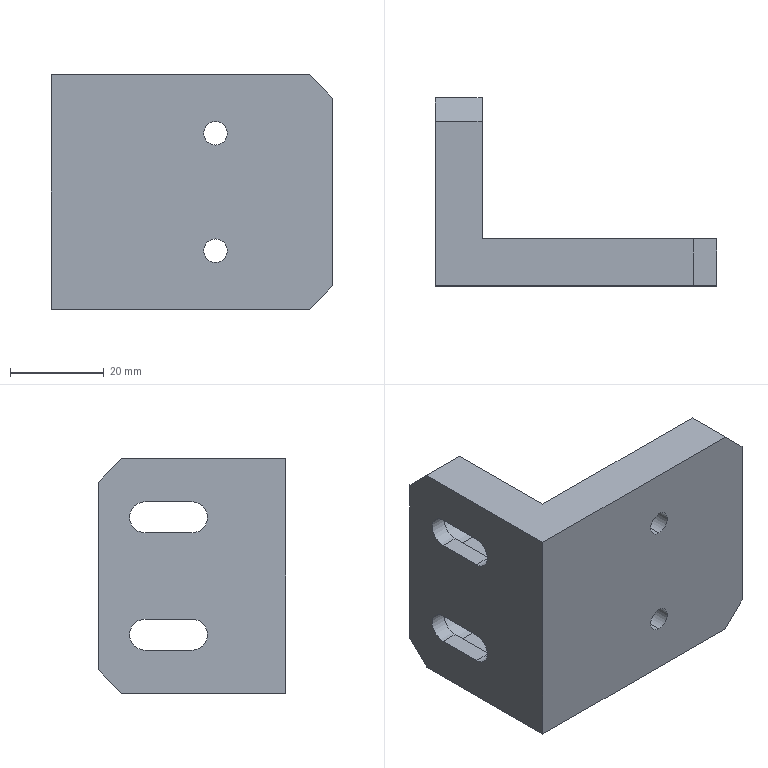Part | SolidWorks | features HoleWzd 2, Chamfer 1, Extrusion 1 | 1 solid | 34 faces | box 60 x 40 x 50 mm | volume 40761 mm3 | plane 22 | cylinder 12 | commonest cylinder face diameters 5 x4 6.6 x4 11 x4
STEP:
#1=CARTESIAN_POINT('',(25.,-10.,35.));
#2=VERTEX_POINT('',#1);
#3=CARTESIAN_POINT('',(25.,-10.,40.));
#4=VERTEX_POINT('',#3);
#5=CARTESIAN_POINT('',(25.,-10.,37.5));
#6=DIRECTION('',(0.,1.,0.));
#7=DIRECTION('',(-1.,0.,0.));
#8=AXIS2_PLACEMENT_3D('',#5,#6,#7);
#9=CIRCLE('',#8,2.5);
#10=EDGE_CURVE('',#2,#4,#9,.T.);
#11=ORIENTED_EDGE('',*,*,#10,.F.);
#12=CARTESIAN_POINT('',(25.,0.,35.));
#13=VERTEX_POINT('',#12);
#14=CARTESIAN_POINT('',(25.,0.,35.));
#15=DIRECTION('',(0.,1.,0.));
#16=VECTOR('',#15,1000.);
#17=LINE('',#14,#16);
#18=EDGE_CURVE('',#2,#13,#17,.T.);
#19=ORIENTED_EDGE('',*,*,#18,.T.);
#20=CARTESIAN_POINT('',(25.,0.,40.));
#21=VERTEX_POINT('',#20);
#22=CARTESIAN_POINT('',(25.,0.,37.5));
#23=DIRECTION('',(0.,1.,0.));
#24=DIRECTION('',(0.,0.,1.));
#25=AXIS2_PLACEMENT_3D('',#22,#23,#24);
#26=CIRCLE('',#25,2.5);
#27=EDGE_CURVE('',#13,#21,#26,.T.);
#28=ORIENTED_EDGE('',*,*,#27,.T.);
#29=CARTESIAN_POINT('',(25.,0.,40.));
#30=DIRECTION('',(0.,1.,0.));
#31=VECTOR('',#30,1000.);
#32=LINE('',#29,#31);
#33=EDGE_CURVE('',#4,#21,#32,.T.);
#34=ORIENTED_EDGE('',*,*,#33,.F.);
#35=EDGE_LOOP('',(#11,#19,#28,#34));
#36=FACE_OUTER_BOUND('',#35,.T.);
#37=CARTESIAN_POINT('',(25.,0.,37.5));
#38=DIRECTION('',(0.,1.,0.));
#39=DIRECTION('',(0.,0.,1.));
#40=AXIS2_PLACEMENT_3D('',#37,#38,#39);
#41=CYLINDRICAL_SURFACE('',#40,2.5);
#42=ADVANCED_FACE('',(#36),#41,.F.);
#43=CARTESIAN_POINT('',(25.,-10.,10.));
#44=VERTEX_POINT('',#43);
#45=CARTESIAN_POINT('',(25.,-10.,15.));
#46=VERTEX_POINT('',#45);
#47=CARTESIAN_POINT('',(25.,-10.,12.5));
#48=DIRECTION('',(0.,1.,0.));
#49=DIRECTION('',(-1.,0.,0.));
#50=AXIS2_PLACEMENT_3D('',#47,#48,#49);
#51=CIRCLE('',#50,2.5);
#52=EDGE_CURVE('',#44,#46,#51,.T.);
#53=ORIENTED_EDGE('',*,*,#52,.F.);
#54=CARTESIAN_POINT('',(25.,0.,10.));
#55=VERTEX_POINT('',#54);
#56=CARTESIAN_POINT('',(25.,0.,10.));
#57=DIRECTION('',(0.,1.,0.));
#58=VECTOR('',#57,1000.);
#59=LINE('',#56,#58);
#60=EDGE_CURVE('',#44,#55,#59,.T.);
#61=ORIENTED_EDGE('',*,*,#60,.T.);
#62=CARTESIAN_POINT('',(25.,0.,15.));
#63=VERTEX_POINT('',#62);
#64=CARTESIAN_POINT('',(25.,0.,12.5));
#65=DIRECTION('',(0.,1.,0.));
#66=DIRECTION('',(0.,0.,1.));
#67=AXIS2_PLACEMENT_3D('',#64,#65,#66);
#68=CIRCLE('',#67,2.5);
#69=EDGE_CURVE('',#55,#63,#68,.T.);
#70=ORIENTED_EDGE('',*,*,#69,.T.);
#71=CARTESIAN_POINT('',(25.,0.,15.));
#72=DIRECTION('',(0.,1.,0.));
#73=VECTOR('',#72,1000.);
#74=LINE('',#71,#73);
#75=EDGE_CURVE('',#46,#63,#74,.T.);
#76=ORIENTED_EDGE('',*,*,#75,.F.);
#77=EDGE_LOOP('',(#53,#61,#70,#76));
#78=FACE_OUTER_BOUND('',#77,.T.);
#79=CARTESIAN_POINT('',(25.,0.,12.5));
#80=DIRECTION('',(0.,1.,0.));
#81=DIRECTION('',(0.,0.,1.));
#82=AXIS2_PLACEMENT_3D('',#79,#80,#81);
#83=CYLINDRICAL_SURFACE('',#82,2.5);
#84=ADVANCED_FACE('',(#78),#83,.F.);
#85=CARTESIAN_POINT('',(0.,10.,32.));
#86=VERTEX_POINT('',#85);
#87=CARTESIAN_POINT('',(0.,20.,32.));
#88=VERTEX_POINT('',#87);
#89=CARTESIAN_POINT('',(0.,10.,32.));
#90=DIRECTION('',(0.,1.,0.));
#91=VECTOR('',#90,1000.);
#92=LINE('',#89,#91);
#93=EDGE_CURVE('',#86,#88,#92,.T.);
#94=ORIENTED_EDGE('',*,*,#93,.F.);
#95=CARTESIAN_POINT('',(0.,10.,43.));
#96=VERTEX_POINT('',#95);
#97=CARTESIAN_POINT('',(0.,10.,37.5));
#98=DIRECTION('',(1.,0.,0.));
#99=DIRECTION('',(0.,0.,-1.));
#100=AXIS2_PLACEMENT_3D('',#97,#98,#99);
#101=CIRCLE('',#100,5.5);
#102=EDGE_CURVE('',#96,#86,#101,.T.);
#103=ORIENTED_EDGE('',*,*,#102,.F.);
#104=CARTESIAN_POINT('',(0.,20.,43.));
#105=VERTEX_POINT('',#104);
#106=CARTESIAN_POINT('',(0.,10.,43.));
#107=DIRECTION('',(0.,1.,0.));
#108=VECTOR('',#107,1000.);
#109=LINE('',#106,#108);
#110=EDGE_CURVE('',#96,#105,#109,.T.);
#111=ORIENTED_EDGE('',*,*,#110,.T.);
#112=CARTESIAN_POINT('',(0.,20.,37.5));
#113=DIRECTION('',(1.,0.,0.));
#114=DIRECTION('',(0.,0.,-1.));
#115=AXIS2_PLACEMENT_3D('',#112,#113,#114);
#116=CIRCLE('',#115,5.5);
#117=EDGE_CURVE('',#88,#105,#116,.T.);
#118=ORIENTED_EDGE('',*,*,#117,.F.);
#119=EDGE_LOOP('',(#94,#103,#111,#118));
#120=FACE_BOUND('',#119,.T.);
#121=CARTESIAN_POINT('',(0.,30.,45.));
#122=VERTEX_POINT('',#121);
#123=CARTESIAN_POINT('',(0.,30.,5.));
#124=VERTEX_POINT('',#123);
#125=CARTESIAN_POINT('',(0.,30.,50.));
#126=DIRECTION('',(0.,0.,-1.));
#127=VECTOR('',#126,1000.);
#128=LINE('',#125,#127);
#129=EDGE_CURVE('',#122,#124,#128,.T.);
#130=ORIENTED_EDGE('',*,*,#129,.F.);
#131=CARTESIAN_POINT('',(0.,25.,50.));
#132=VERTEX_POINT('',#131);
#133=CARTESIAN_POINT('',(0.,25.,50.));
#134=DIRECTION('',(0.,-0.7071,0.7071));
#135=VECTOR('',#134,1000.);
#136=LINE('',#133,#135);
#137=EDGE_CURVE('',#122,#132,#136,.T.);
#138=ORIENTED_EDGE('',*,*,#137,.T.);
#139=CARTESIAN_POINT('',(0.,0.,50.));
#140=VERTEX_POINT('',#139);
#141=CARTESIAN_POINT('',(0.,0.,50.));
#142=DIRECTION('',(0.,1.,0.));
#143=VECTOR('',#142,1000.);
#144=LINE('',#141,#143);
#145=EDGE_CURVE('',#140,#132,#144,.T.);
#146=ORIENTED_EDGE('',*,*,#145,.F.);
#147=CARTESIAN_POINT('',(0.,0.,0.));
#148=VERTEX_POINT('',#147);
#149=CARTESIAN_POINT('',(0.,0.,50.));
#150=DIRECTION('',(0.,0.,-1.));
#151=VECTOR('',#150,1000.);
#152=LINE('',#149,#151);
#153=EDGE_CURVE('',#140,#148,#152,.T.);
#154=ORIENTED_EDGE('',*,*,#153,.T.);
#155=CARTESIAN_POINT('',(0.,25.,0.));
#156=VERTEX_POINT('',#155);
#157=CARTESIAN_POINT('',(0.,0.,0.));
#158=DIRECTION('',(0.,1.,0.));
#159=VECTOR('',#158,1000.);
#160=LINE('',#157,#159);
#161=EDGE_CURVE('',#148,#156,#160,.T.);
#162=ORIENTED_EDGE('',*,*,#161,.T.);
#163=CARTESIAN_POINT('',(0.,30.,5.));
#164=DIRECTION('',(0.,0.7071,0.7071));
#165=VECTOR('',#164,1000.);
#166=LINE('',#163,#165);
#167=EDGE_CURVE('',#156,#124,#166,.T.);
#168=ORIENTED_EDGE('',*,*,#167,.T.);
#169=EDGE_LOOP('',(#130,#138,#146,#154,#162,#168));
#170=FACE_OUTER_BOUND('',#169,.T.);
#171=CARTESIAN_POINT('',(0.,10.,7.));
#172=VERTEX_POINT('',#171);
#173=CARTESIAN_POINT('',(0.,20.,7.));
#174=VERTEX_POINT('',#173);
#175=CARTESIAN_POINT('',(0.,10.,7.));
#176=DIRECTION('',(0.,1.,0.));
#177=VECTOR('',#176,1000.);
#178=LINE('',#175,#177);
#179=EDGE_CURVE('',#172,#174,#178,.T.);
#180=ORIENTED_EDGE('',*,*,#179,.F.);
#181=CARTESIAN_POINT('',(0.,10.,18.));
#182=VERTEX_POINT('',#181);
#183=CARTESIAN_POINT('',(0.,10.,12.5));
#184=DIRECTION('',(1.,0.,0.));
#185=DIRECTION('',(0.,0.,-1.));
#186=AXIS2_PLACEMENT_3D('',#183,#184,#185);
#187=CIRCLE('',#186,5.5);
#188=EDGE_CURVE('',#182,#172,#187,.T.);
#189=ORIENTED_EDGE('',*,*,#188,.F.);
#190=CARTESIAN_POINT('',(0.,20.,18.));
#191=VERTEX_POINT('',#190);
#192=CARTESIAN_POINT('',(0.,10.,18.));
#193=DIRECTION('',(0.,1.,0.));
#194=VECTOR('',#193,1000.);
#195=LINE('',#192,#194);
#196=EDGE_CURVE('',#182,#191,#195,.T.);
#197=ORIENTED_EDGE('',*,*,#196,.T.);
#198=CARTESIAN_POINT('',(0.,20.,12.5));
#199=DIRECTION('',(1.,0.,0.));
#200=DIRECTION('',(0.,0.,-1.));
#201=AXIS2_PLACEMENT_3D('',#198,#199,#200);
#202=CIRCLE('',#201,5.5);
#203=EDGE_CURVE('',#174,#191,#202,.T.);
#204=ORIENTED_EDGE('',*,*,#203,.F.);
#205=EDGE_LOOP('',(#180,#189,#197,#204));
#206=FACE_BOUND('',#205,.T.);
#207=CARTESIAN_POINT('',(0.,0.,50.));
#208=DIRECTION('',(-1.,0.,0.));
#209=DIRECTION('',(0.,-1.,0.));
#210=AXIS2_PLACEMENT_3D('',#207,#208,#209);
#211=PLANE('',#210);
#212=ADVANCED_FACE('',(#120,#170,#206),#211,.F.);
#213=CARTESIAN_POINT('',(50.,-10.,45.));
#214=VERTEX_POINT('',#213);
#215=CARTESIAN_POINT('',(50.,-10.,5.));
#216=VERTEX_POINT('',#215);
#217=CARTESIAN_POINT('',(50.,-10.,50.));
#218=DIRECTION('',(0.,0.,-1.));
#219=VECTOR('',#218,1000.);
#220=LINE('',#217,#219);
#221=EDGE_CURVE('',#214,#216,#220,.T.);
#222=ORIENTED_EDGE('',*,*,#221,.T.);
#223=CARTESIAN_POINT('',(50.,0.,5.));
#224=VERTEX_POINT('',#223);
#225=CARTESIAN_POINT('',(50.,0.,5.));
#226=DIRECTION('',(0.,1.,0.));
#227=VECTOR('',#226,1000.);
#228=LINE('',#225,#227);
#229=EDGE_CURVE('',#216,#224,#228,.T.);
#230=ORIENTED_EDGE('',*,*,#229,.T.);
#231=CARTESIAN_POINT('',(50.,0.,45.));
#232=VERTEX_POINT('',#231);
#233=CARTESIAN_POINT('',(50.,0.,50.));
#234=DIRECTION('',(0.,0.,-1.));
#235=VECTOR('',#234,1000.);
#236=LINE('',#233,#235);
#237=EDGE_CURVE('',#232,#224,#236,.T.);
#238=ORIENTED_EDGE('',*,*,#237,.F.);
#239=CARTESIAN_POINT('',(50.,0.,45.));
#240=DIRECTION('',(0.,-1.,0.));
#241=VECTOR('',#240,1000.);
#242=LINE('',#239,#241);
#243=EDGE_CURVE('',#232,#214,#242,.T.);
#244=ORIENTED_EDGE('',*,*,#243,.T.);
#245=EDGE_LOOP('',(#222,#230,#238,#244));
#246=FACE_OUTER_BOUND('',#245,.T.);
#247=CARTESIAN_POINT('',(50.,0.,50.));
#248=DIRECTION('',(-1.,0.,0.));
#249=DIRECTION('',(0.,0.,1.));
#250=AXIS2_PLACEMENT_3D('',#247,#248,#249);
#251=PLANE('',#250);
#252=ADVANCED_FACE('',(#246),#251,.F.);
#253=CARTESIAN_POINT('',(25.,0.,37.5));
#254=DIRECTION('',(0.,1.,0.));
#255=DIRECTION('',(0.,0.,1.));
#256=AXIS2_PLACEMENT_3D('',#253,#254,#255);
#257=CIRCLE('',#256,2.5);
#258=EDGE_CURVE('',#21,#13,#257,.T.);
#259=ORIENTED_EDGE('',*,*,#258,.F.);
#260=ORIENTED_EDGE('',*,*,#27,.F.);
#261=EDGE_LOOP('',(#259,#260));
#262=FACE_BOUND('',#261,.T.);
#263=CARTESIAN_POINT('',(25.,0.,12.5));
#264=DIRECTION('',(0.,1.,0.));
#265=DIRECTION('',(0.,0.,1.));
#266=AXIS2_PLACEMENT_3D('',#263,#264,#265);
#267=CIRCLE('',#266,2.5);
#268=EDGE_CURVE('',#63,#55,#267,.T.);
#269=ORIENTED_EDGE('',*,*,#268,.F.);
#270=ORIENTED_EDGE('',*,*,#69,.F.);
#271=EDGE_LOOP('',(#269,#270));
#272=FACE_BOUND('',#271,.T.);
#273=ORIENTED_EDGE('',*,*,#237,.T.);
#274=CARTESIAN_POINT('',(45.,0.,0.));
#275=VERTEX_POINT('',#274);
#276=CARTESIAN_POINT('',(50.,0.,5.));
#277=DIRECTION('',(-0.7071,0.,-0.7071));
#278=VECTOR('',#277,1000.);
#279=LINE('',#276,#278);
#280=EDGE_CURVE('',#224,#275,#279,.T.);
#281=ORIENTED_EDGE('',*,*,#280,.T.);
#282=CARTESIAN_POINT('',(50.,0.,0.));
#283=DIRECTION('',(-1.,0.,0.));
#284=VECTOR('',#283,1000.);
#285=LINE('',#282,#284);
#286=EDGE_CURVE('',#275,#148,#285,.T.);
#287=ORIENTED_EDGE('',*,*,#286,.T.);
#288=ORIENTED_EDGE('',*,*,#153,.F.);
#289=CARTESIAN_POINT('',(45.,0.,50.));
#290=VERTEX_POINT('',#289);
#291=CARTESIAN_POINT('',(50.,0.,50.));
#292=DIRECTION('',(-1.,0.,0.));
#293=VECTOR('',#292,1000.);
#294=LINE('',#291,#293);
#295=EDGE_CURVE('',#290,#140,#294,.T.);
#296=ORIENTED_EDGE('',*,*,#295,.F.);
#297=CARTESIAN_POINT('',(45.,0.,50.));
#298=DIRECTION('',(0.7071,0.,-0.7071));
#299=VECTOR('',#298,1000.);
#300=LINE('',#297,#299);
#301=EDGE_CURVE('',#290,#232,#300,.T.);
#302=ORIENTED_EDGE('',*,*,#301,.T.);
#303=EDGE_LOOP('',(#273,#281,#287,#288,#296,#302));
#304=FACE_OUTER_BOUND('',#303,.T.);
#305=CARTESIAN_POINT('',(50.,0.,50.));
#306=DIRECTION('',(0.,-1.,0.));
#307=DIRECTION('',(1.,0.,0.));
#308=AXIS2_PLACEMENT_3D('',#305,#306,#307);
#309=PLANE('',#308);
#310=ADVANCED_FACE('',(#262,#272,#304),#309,.F.);
#311=CARTESIAN_POINT('',(-10.,30.,45.));
#312=VERTEX_POINT('',#311);
#313=CARTESIAN_POINT('',(-10.,30.,5.));
#314=VERTEX_POINT('',#313);
#315=CARTESIAN_POINT('',(-10.,30.,50.));
#316=DIRECTION('',(0.,0.,-1.));
#317=VECTOR('',#316,1000.);
#318=LINE('',#315,#317);
#319=EDGE_CURVE('',#312,#314,#318,.T.);
#320=ORIENTED_EDGE('',*,*,#319,.F.);
#321=CARTESIAN_POINT('',(-10.,30.,45.));
#322=DIRECTION('',(1.,0.,0.));
#323=VECTOR('',#322,1000.);
#324=LINE('',#321,#323);
#325=EDGE_CURVE('',#312,#122,#324,.T.);
#326=ORIENTED_EDGE('',*,*,#325,.T.);
#327=ORIENTED_EDGE('',*,*,#129,.T.);
#328=CARTESIAN_POINT('',(-10.,30.,5.));
#329=DIRECTION('',(-1.,0.,0.));
#330=VECTOR('',#329,1000.);
#331=LINE('',#328,#330);
#332=EDGE_CURVE('',#124,#314,#331,.T.);
#333=ORIENTED_EDGE('',*,*,#332,.T.);
#334=EDGE_LOOP('',(#320,#326,#327,#333));
#335=FACE_OUTER_BOUND('',#334,.T.);
#336=CARTESIAN_POINT('',(-10.,30.,50.));
#337=DIRECTION('',(0.,-1.,0.));
#338=DIRECTION('',(1.,0.,0.));
#339=AXIS2_PLACEMENT_3D('',#336,#337,#338);
#340=PLANE('',#339);
#341=ADVANCED_FACE('',(#335),#340,.F.);
#342=CARTESIAN_POINT('',(-10.,10.,34.2));
#343=VERTEX_POINT('',#342);
#344=CARTESIAN_POINT('',(-10.,20.,34.2));
#345=VERTEX_POINT('',#344);
#346=CARTESIAN_POINT('',(-10.,-10.,34.2));
#347=DIRECTION('',(0.,1.,0.));
#348=VECTOR('',#347,1000.);
#349=LINE('',#346,#348);
#350=EDGE_CURVE('',#343,#345,#349,.T.);
#351=ORIENTED_EDGE('',*,*,#350,.T.);
#352=CARTESIAN_POINT('',(-10.,20.,40.8));
#353=VERTEX_POINT('',#352);
#354=CARTESIAN_POINT('',(-10.,20.,37.5));
#355=DIRECTION('',(1.,0.,0.));
#356=DIRECTION('',(0.,1.,0.));
#357=AXIS2_PLACEMENT_3D('',#354,#355,#356);
#358=CIRCLE('',#357,3.3);
#359=EDGE_CURVE('',#345,#353,#358,.T.);
#360=ORIENTED_EDGE('',*,*,#359,.T.);
#361=CARTESIAN_POINT('',(-10.,10.,40.8));
#362=VERTEX_POINT('',#361);
#363=CARTESIAN_POINT('',(-10.,-10.,40.8));
#364=DIRECTION('',(0.,-1.,0.));
#365=VECTOR('',#364,1000.);
#366=LINE('',#363,#365);
#367=EDGE_CURVE('',#353,#362,#366,.T.);
#368=ORIENTED_EDGE('',*,*,#367,.T.);
#369=CARTESIAN_POINT('',(-10.,10.,37.5));
#370=DIRECTION('',(1.,0.,0.));
#371=DIRECTION('',(0.,1.,0.));
#372=AXIS2_PLACEMENT_3D('',#369,#370,#371);
#373=CIRCLE('',#372,3.3);
#374=EDGE_CURVE('',#362,#343,#373,.T.);
#375=ORIENTED_EDGE('',*,*,#374,.T.);
#376=EDGE_LOOP('',(#351,#360,#368,#375));
#377=FACE_BOUND('',#376,.T.);
#378=CARTESIAN_POINT('',(-10.,20.,15.8));
#379=VERTEX_POINT('',#378);
#380=CARTESIAN_POINT('',(-10.,10.,15.8));
#381=VERTEX_POINT('',#380);
#382=CARTESIAN_POINT('',(-10.,-10.,15.8));
#383=DIRECTION('',(0.,-1.,0.));
#384=VECTOR('',#383,1000.);
#385=LINE('',#382,#384);
#386=EDGE_CURVE('',#379,#381,#385,.T.);
#387=ORIENTED_EDGE('',*,*,#386,.T.);
#388=CARTESIAN_POINT('',(-10.,10.,9.2));
#389=VERTEX_POINT('',#388);
#390=CARTESIAN_POINT('',(-10.,10.,12.5));
#391=DIRECTION('',(1.,0.,0.));
#392=DIRECTION('',(0.,1.,0.));
#393=AXIS2_PLACEMENT_3D('',#390,#391,#392);
#394=CIRCLE('',#393,3.3);
#395=EDGE_CURVE('',#381,#389,#394,.T.);
#396=ORIENTED_EDGE('',*,*,#395,.T.);
#397=CARTESIAN_POINT('',(-10.,20.,9.2));
#398=VERTEX_POINT('',#397);
#399=CARTESIAN_POINT('',(-10.,-10.,9.2));
#400=DIRECTION('',(0.,1.,0.));
#401=VECTOR('',#400,1000.);
#402=LINE('',#399,#401);
#403=EDGE_CURVE('',#389,#398,#402,.T.);
#404=ORIENTED_EDGE('',*,*,#403,.T.);
#405=CARTESIAN_POINT('',(-10.,20.,12.5));
#406=DIRECTION('',(1.,0.,0.));
#407=DIRECTION('',(0.,1.,0.));
#408=AXIS2_PLACEMENT_3D('',#405,#406,#407);
#409=CIRCLE('',#408,3.3);
#410=EDGE_CURVE('',#398,#379,#409,.T.);
#411=ORIENTED_EDGE('',*,*,#410,.T.);
#412=EDGE_LOOP('',(#387,#396,#404,#411));
#413=FACE_BOUND('',#412,.T.);
#414=CARTESIAN_POINT('',(-10.,25.,50.));
#415=VERTEX_POINT('',#414);
#416=CARTESIAN_POINT('',(-10.,-10.,50.));
#417=VERTEX_POINT('',#416);
#418=CARTESIAN_POINT('',(-10.,-10.,50.));
#419=DIRECTION('',(0.,-1.,0.));
#420=VECTOR('',#419,1000.);
#421=LINE('',#418,#420);
#422=EDGE_CURVE('',#415,#417,#421,.T.);
#423=ORIENTED_EDGE('',*,*,#422,.F.);
#424=CARTESIAN_POINT('',(-10.,25.,50.));
#425=DIRECTION('',(0.,0.7071,-0.7071));
#426=VECTOR('',#425,1000.);
#427=LINE('',#424,#426);
#428=EDGE_CURVE('',#415,#312,#427,.T.);
#429=ORIENTED_EDGE('',*,*,#428,.T.);
#430=ORIENTED_EDGE('',*,*,#319,.T.);
#431=CARTESIAN_POINT('',(-10.,25.,0.));
#432=VERTEX_POINT('',#431);
#433=CARTESIAN_POINT('',(-10.,30.,5.));
#434=DIRECTION('',(0.,-0.7071,-0.7071));
#435=VECTOR('',#434,1000.);
#436=LINE('',#433,#435);
#437=EDGE_CURVE('',#314,#432,#436,.T.);
#438=ORIENTED_EDGE('',*,*,#437,.T.);
#439=CARTESIAN_POINT('',(-10.,-10.,0.));
#440=VERTEX_POINT('',#439);
#441=CARTESIAN_POINT('',(-10.,-10.,0.));
#442=DIRECTION('',(0.,-1.,0.));
#443=VECTOR('',#442,1000.);
#444=LINE('',#441,#443);
#445=EDGE_CURVE('',#432,#440,#444,.T.);
#446=ORIENTED_EDGE('',*,*,#445,.T.);
#447=CARTESIAN_POINT('',(-10.,-10.,50.));
#448=DIRECTION('',(0.,0.,-1.));
#449=VECTOR('',#448,1000.);
#450=LINE('',#447,#449);
#451=EDGE_CURVE('',#417,#440,#450,.T.);
#452=ORIENTED_EDGE('',*,*,#451,.F.);
#453=EDGE_LOOP('',(#423,#429,#430,#438,#446,#452));
#454=FACE_OUTER_BOUND('',#453,.T.);
#455=CARTESIAN_POINT('',(-10.,-10.,50.));
#456=DIRECTION('',(1.,0.,0.));
#457=DIRECTION('',(0.,1.,0.));
#458=AXIS2_PLACEMENT_3D('',#455,#456,#457);
#459=PLANE('',#458);
#460=ADVANCED_FACE('',(#377,#413,#454),#459,.F.);
#461=CARTESIAN_POINT('',(25.,-10.,37.5));
#462=DIRECTION('',(0.,1.,0.));
#463=DIRECTION('',(-1.,0.,0.));
#464=AXIS2_PLACEMENT_3D('',#461,#462,#463);
#465=CIRCLE('',#464,2.5);
#466=EDGE_CURVE('',#4,#2,#465,.T.);
#467=ORIENTED_EDGE('',*,*,#466,.T.);
#468=ORIENTED_EDGE('',*,*,#10,.T.);
#469=EDGE_LOOP('',(#467,#468));
#470=FACE_BOUND('',#469,.T.);
#471=CARTESIAN_POINT('',(25.,-10.,12.5));
#472=DIRECTION('',(0.,1.,0.));
#473=DIRECTION('',(-1.,0.,0.));
#474=AXIS2_PLACEMENT_3D('',#471,#472,#473);
#475=CIRCLE('',#474,2.5);
#476=EDGE_CURVE('',#46,#44,#475,.T.);
#477=ORIENTED_EDGE('',*,*,#476,.T.);
#478=ORIENTED_EDGE('',*,*,#52,.T.);
#479=EDGE_LOOP('',(#477,#478));
#480=FACE_BOUND('',#479,.T.);
#481=CARTESIAN_POINT('',(45.,-10.,0.));
#482=VERTEX_POINT('',#481);
#483=CARTESIAN_POINT('',(50.,-10.,0.));
#484=DIRECTION('',(1.,0.,0.));
#485=VECTOR('',#484,1000.);
#486=LINE('',#483,#485);
#487=EDGE_CURVE('',#440,#482,#486,.T.);
#488=ORIENTED_EDGE('',*,*,#487,.T.);
#489=CARTESIAN_POINT('',(50.,-10.,5.));
#490=DIRECTION('',(0.7071,0.,0.7071));
#491=VECTOR('',#490,1000.);
#492=LINE('',#489,#491);
#493=EDGE_CURVE('',#482,#216,#492,.T.);
#494=ORIENTED_EDGE('',*,*,#493,.T.);
#495=ORIENTED_EDGE('',*,*,#221,.F.);
#496=CARTESIAN_POINT('',(45.,-10.,50.));
#497=VERTEX_POINT('',#496);
#498=CARTESIAN_POINT('',(45.,-10.,50.));
#499=DIRECTION('',(-0.7071,0.,0.7071));
#500=VECTOR('',#499,1000.);
#501=LINE('',#498,#500);
#502=EDGE_CURVE('',#214,#497,#501,.T.);
#503=ORIENTED_EDGE('',*,*,#502,.T.);
#504=CARTESIAN_POINT('',(50.,-10.,50.));
#505=DIRECTION('',(1.,0.,0.));
#506=VECTOR('',#505,1000.);
#507=LINE('',#504,#506);
#508=EDGE_CURVE('',#417,#497,#507,.T.);
#509=ORIENTED_EDGE('',*,*,#508,.F.);
#510=ORIENTED_EDGE('',*,*,#451,.T.);
#511=EDGE_LOOP('',(#488,#494,#495,#503,#509,#510));
#512=FACE_OUTER_BOUND('',#511,.T.);
#513=CARTESIAN_POINT('',(50.,-10.,50.));
#514=DIRECTION('',(0.,1.,0.));
#515=DIRECTION('',(-1.,0.,0.));
#516=AXIS2_PLACEMENT_3D('',#513,#514,#515);
#517=PLANE('',#516);
#518=ADVANCED_FACE('',(#470,#480,#512),#517,.F.);
#519=ORIENTED_EDGE('',*,*,#508,.T.);
#520=CARTESIAN_POINT('',(45.,0.,50.));
#521=DIRECTION('',(0.,1.,0.));
#522=VECTOR('',#521,1000.);
#523=LINE('',#520,#522);
#524=EDGE_CURVE('',#497,#290,#523,.T.);
#525=ORIENTED_EDGE('',*,*,#524,.T.);
#526=ORIENTED_EDGE('',*,*,#295,.T.);
#527=ORIENTED_EDGE('',*,*,#145,.T.);
#528=CARTESIAN_POINT('',(0.,25.,50.));
#529=DIRECTION('',(-1.,0.,0.));
#530=VECTOR('',#529,1000.);
#531=LINE('',#528,#530);
#532=EDGE_CURVE('',#132,#415,#531,.T.);
#533=ORIENTED_EDGE('',*,*,#532,.T.);
#534=ORIENTED_EDGE('',*,*,#422,.T.);
#535=EDGE_LOOP('',(#519,#525,#526,#527,#533,#534));
#536=FACE_OUTER_BOUND('',#535,.T.);
#537=CARTESIAN_POINT('',(0.,0.,50.));
#538=DIRECTION('',(0.,0.,-1.));
#539=DIRECTION('',(-1.,0.,0.));
#540=AXIS2_PLACEMENT_3D('',#537,#538,#539);
#541=PLANE('',#540);
#542=ADVANCED_FACE('',(#536),#541,.F.);
#543=ORIENTED_EDGE('',*,*,#286,.F.);
#544=CARTESIAN_POINT('',(45.,-10.,0.));
#545=DIRECTION('',(0.,-1.,0.));
#546=VECTOR('',#545,1000.);
#547=LINE('',#544,#546);
#548=EDGE_CURVE('',#275,#482,#547,.T.);
#549=ORIENTED_EDGE('',*,*,#548,.T.);
#550=ORIENTED_EDGE('',*,*,#487,.F.);
#551=ORIENTED_EDGE('',*,*,#445,.F.);
#552=CARTESIAN_POINT('',(0.,25.,0.));
#553=DIRECTION('',(1.,0.,0.));
#554=VECTOR('',#553,1000.);
#555=LINE('',#552,#554);
#556=EDGE_CURVE('',#432,#156,#555,.T.);
#557=ORIENTED_EDGE('',*,*,#556,.T.);
#558=ORIENTED_EDGE('',*,*,#161,.F.);
#559=EDGE_LOOP('',(#543,#549,#550,#551,#557,#558));
#560=FACE_OUTER_BOUND('',#559,.T.);
#561=CARTESIAN_POINT('',(0.,0.,0.));
#562=DIRECTION('',(0.,0.,-1.));
#563=DIRECTION('',(-1.,0.,0.));
#564=AXIS2_PLACEMENT_3D('',#561,#562,#563);
#565=PLANE('',#564);
#566=ADVANCED_FACE('',(#560),#565,.T.);
#567=CARTESIAN_POINT('',(-6.4,10.,15.8));
#568=VERTEX_POINT('',#567);
#569=CARTESIAN_POINT('',(0.,10.,15.8));
#570=DIRECTION('',(-1.,0.,0.));
#571=VECTOR('',#570,1000.);
#572=LINE('',#569,#571);
#573=EDGE_CURVE('',#568,#381,#572,.T.);
#574=ORIENTED_EDGE('',*,*,#573,.F.);
#575=CARTESIAN_POINT('',(-6.4,10.,9.2));
#576=VERTEX_POINT('',#575);
#577=CARTESIAN_POINT('',(-6.4,10.,12.5));
#578=DIRECTION('',(1.,0.,0.));
#579=DIRECTION('',(0.,0.,-1.));
#580=AXIS2_PLACEMENT_3D('',#577,#578,#579);
#581=CIRCLE('',#580,3.3);
#582=EDGE_CURVE('',#568,#576,#581,.T.);
#583=ORIENTED_EDGE('',*,*,#582,.T.);
#584=CARTESIAN_POINT('',(0.,10.,9.2));
#585=DIRECTION('',(1.,0.,0.));
#586=VECTOR('',#585,1000.);
#587=LINE('',#584,#586);
#588=EDGE_CURVE('',#389,#576,#587,.T.);
#589=ORIENTED_EDGE('',*,*,#588,.F.);
#590=ORIENTED_EDGE('',*,*,#395,.F.);
#591=EDGE_LOOP('',(#574,#583,#589,#590));
#592=FACE_OUTER_BOUND('',#591,.T.);
#593=CARTESIAN_POINT('',(0.,10.,12.5));
#594=DIRECTION('',(1.,0.,0.));
#595=DIRECTION('',(0.,0.,-1.));
#596=AXIS2_PLACEMENT_3D('',#593,#594,#595);
#597=CYLINDRICAL_SURFACE('',#596,3.3);
#598=ADVANCED_FACE('',(#592),#597,.F.);
#599=CARTESIAN_POINT('',(-6.4,20.,15.8));
#600=VERTEX_POINT('',#599);
#601=CARTESIAN_POINT('',(0.,20.,15.8));
#602=DIRECTION('',(1.,0.,0.));
#603=VECTOR('',#602,1000.);
#604=LINE('',#601,#603);
#605=EDGE_CURVE('',#379,#600,#604,.T.);
#606=ORIENTED_EDGE('',*,*,#605,.T.);
#607=CARTESIAN_POINT('',(-6.4,10.,15.8));
#608=DIRECTION('',(0.,1.,0.));
#609=VECTOR('',#608,1000.);
#610=LINE('',#607,#609);
#611=EDGE_CURVE('',#568,#600,#610,.T.);
#612=ORIENTED_EDGE('',*,*,#611,.F.);
#613=ORIENTED_EDGE('',*,*,#573,.T.);
#614=ORIENTED_EDGE('',*,*,#386,.F.);
#615=EDGE_LOOP('',(#606,#612,#613,#614));
#616=FACE_OUTER_BOUND('',#615,.T.);
#617=CARTESIAN_POINT('',(0.,10.,15.8));
#618=DIRECTION('',(0.,0.,1.));
#619=DIRECTION('',(1.,0.,0.));
#620=AXIS2_PLACEMENT_3D('',#617,#618,#619);
#621=PLANE('',#620);
#622=ADVANCED_FACE('',(#616),#621,.F.);
#623=CARTESIAN_POINT('',(-6.4,20.,9.2));
#624=VERTEX_POINT('',#623);
#625=CARTESIAN_POINT('',(0.,20.,9.2));
#626=DIRECTION('',(-1.,0.,0.));
#627=VECTOR('',#626,1000.);
#628=LINE('',#625,#627);
#629=EDGE_CURVE('',#624,#398,#628,.T.);
#630=ORIENTED_EDGE('',*,*,#629,.F.);
#631=CARTESIAN_POINT('',(-6.4,20.,12.5));
#632=DIRECTION('',(1.,0.,0.));
#633=DIRECTION('',(0.,0.,-1.));
#634=AXIS2_PLACEMENT_3D('',#631,#632,#633);
#635=CIRCLE('',#634,3.3);
#636=EDGE_CURVE('',#624,#600,#635,.T.);
#637=ORIENTED_EDGE('',*,*,#636,.T.);
#638=ORIENTED_EDGE('',*,*,#605,.F.);
#639=ORIENTED_EDGE('',*,*,#410,.F.);
#640=EDGE_LOOP('',(#630,#637,#638,#639));
#641=FACE_OUTER_BOUND('',#640,.T.);
#642=CARTESIAN_POINT('',(0.,20.,12.5));
#643=DIRECTION('',(1.,0.,0.));
#644=DIRECTION('',(0.,0.,-1.));
#645=AXIS2_PLACEMENT_3D('',#642,#643,#644);
#646=CYLINDRICAL_SURFACE('',#645,3.3);
#647=ADVANCED_FACE('',(#641),#646,.F.);
#648=ORIENTED_EDGE('',*,*,#588,.T.);
#649=CARTESIAN_POINT('',(-6.4,10.,9.2));
#650=DIRECTION('',(0.,1.,0.));
#651=VECTOR('',#650,1000.);
#652=LINE('',#649,#651);
#653=EDGE_CURVE('',#576,#624,#652,.T.);
#654=ORIENTED_EDGE('',*,*,#653,.T.);
#655=ORIENTED_EDGE('',*,*,#629,.T.);
#656=ORIENTED_EDGE('',*,*,#403,.F.);
#657=EDGE_LOOP('',(#648,#654,#655,#656));
#658=FACE_OUTER_BOUND('',#657,.T.);
#659=CARTESIAN_POINT('',(0.,10.,9.2));
#660=DIRECTION('',(0.,0.,-1.));
#661=DIRECTION('',(-1.,0.,0.));
#662=AXIS2_PLACEMENT_3D('',#659,#660,#661);
#663=PLANE('',#662);
#664=ADVANCED_FACE('',(#658),#663,.F.);
#665=ORIENTED_EDGE('',*,*,#653,.F.);
#666=ORIENTED_EDGE('',*,*,#582,.F.);
#667=ORIENTED_EDGE('',*,*,#611,.T.);
#668=ORIENTED_EDGE('',*,*,#636,.F.);
#669=EDGE_LOOP('',(#665,#666,#667,#668));
#670=FACE_BOUND('',#669,.T.);
#671=CARTESIAN_POINT('',(-6.4,20.,7.));
#672=VERTEX_POINT('',#671);
#673=CARTESIAN_POINT('',(-6.4,20.,18.));
#674=VERTEX_POINT('',#673);
#675=CARTESIAN_POINT('',(-6.4,20.,12.5));
#676=DIRECTION('',(1.,0.,0.));
#677=DIRECTION('',(0.,0.,-1.));
#678=AXIS2_PLACEMENT_3D('',#675,#676,#677);
#679=CIRCLE('',#678,5.5);
#680=EDGE_CURVE('',#672,#674,#679,.T.);
#681=ORIENTED_EDGE('',*,*,#680,.T.);
#682=CARTESIAN_POINT('',(-6.4,10.,18.));
#683=VERTEX_POINT('',#682);
#684=CARTESIAN_POINT('',(-6.4,10.,18.));
#685=DIRECTION('',(0.,1.,0.));
#686=VECTOR('',#685,1000.);
#687=LINE('',#684,#686);
#688=EDGE_CURVE('',#683,#674,#687,.T.);
#689=ORIENTED_EDGE('',*,*,#688,.F.);
#690=CARTESIAN_POINT('',(-6.4,10.,7.));
#691=VERTEX_POINT('',#690);
#692=CARTESIAN_POINT('',(-6.4,10.,12.5));
#693=DIRECTION('',(1.,0.,0.));
#694=DIRECTION('',(0.,0.,-1.));
#695=AXIS2_PLACEMENT_3D('',#692,#693,#694);
#696=CIRCLE('',#695,5.5);
#697=EDGE_CURVE('',#683,#691,#696,.T.);
#698=ORIENTED_EDGE('',*,*,#697,.T.);
#699=CARTESIAN_POINT('',(-6.4,10.,7.));
#700=DIRECTION('',(0.,1.,0.));
#701=VECTOR('',#700,1000.);
#702=LINE('',#699,#701);
#703=EDGE_CURVE('',#691,#672,#702,.T.);
#704=ORIENTED_EDGE('',*,*,#703,.T.);
#705=EDGE_LOOP('',(#681,#689,#698,#704));
#706=FACE_OUTER_BOUND('',#705,.T.);
#707=CARTESIAN_POINT('',(-6.4,23.3,12.5));
#708=DIRECTION('',(-1.,0.,0.));
#709=DIRECTION('',(0.,0.,1.));
#710=AXIS2_PLACEMENT_3D('',#707,#708,#709);
#711=PLANE('',#710);
#712=ADVANCED_FACE('',(#670,#706),#711,.F.);
#713=ORIENTED_EDGE('',*,*,#680,.F.);
#714=CARTESIAN_POINT('',(0.,20.,7.));
#715=DIRECTION('',(-1.,0.,0.));
#716=VECTOR('',#715,1000.);
#717=LINE('',#714,#716);
#718=EDGE_CURVE('',#174,#672,#717,.T.);
#719=ORIENTED_EDGE('',*,*,#718,.F.);
#720=ORIENTED_EDGE('',*,*,#203,.T.);
#721=CARTESIAN_POINT('',(0.,20.,18.));
#722=DIRECTION('',(1.,0.,0.));
#723=VECTOR('',#722,1000.);
#724=LINE('',#721,#723);
#725=EDGE_CURVE('',#674,#191,#724,.T.);
#726=ORIENTED_EDGE('',*,*,#725,.F.);
#727=EDGE_LOOP('',(#713,#719,#720,#726));
#728=FACE_OUTER_BOUND('',#727,.T.);
#729=CARTESIAN_POINT('',(0.,20.,12.5));
#730=DIRECTION('',(1.,0.,0.));
#731=DIRECTION('',(0.,0.,-1.));
#732=AXIS2_PLACEMENT_3D('',#729,#730,#731);
#733=CYLINDRICAL_SURFACE('',#732,5.5);
#734=ADVANCED_FACE('',(#728),#733,.F.);
#735=ORIENTED_EDGE('',*,*,#188,.T.);
#736=CARTESIAN_POINT('',(0.,10.,7.));
#737=DIRECTION('',(1.,0.,0.));
#738=VECTOR('',#737,1000.);
#739=LINE('',#736,#738);
#740=EDGE_CURVE('',#691,#172,#739,.T.);
#741=ORIENTED_EDGE('',*,*,#740,.F.);
#742=ORIENTED_EDGE('',*,*,#697,.F.);
#743=CARTESIAN_POINT('',(0.,10.,18.));
#744=DIRECTION('',(-1.,0.,0.));
#745=VECTOR('',#744,1000.);
#746=LINE('',#743,#745);
#747=EDGE_CURVE('',#182,#683,#746,.T.);
#748=ORIENTED_EDGE('',*,*,#747,.F.);
#749=EDGE_LOOP('',(#735,#741,#742,#748));
#750=FACE_OUTER_BOUND('',#749,.T.);
#751=CARTESIAN_POINT('',(0.,10.,12.5));
#752=DIRECTION('',(1.,0.,0.));
#753=DIRECTION('',(0.,0.,-1.));
#754=AXIS2_PLACEMENT_3D('',#751,#752,#753);
#755=CYLINDRICAL_SURFACE('',#754,5.5);
#756=ADVANCED_FACE('',(#750),#755,.F.);
#757=ORIENTED_EDGE('',*,*,#725,.T.);
#758=ORIENTED_EDGE('',*,*,#196,.F.);
#759=ORIENTED_EDGE('',*,*,#747,.T.);
#760=ORIENTED_EDGE('',*,*,#688,.T.);
#761=EDGE_LOOP('',(#757,#758,#759,#760));
#762=FACE_OUTER_BOUND('',#761,.T.);
#763=CARTESIAN_POINT('',(0.,10.,18.));
#764=DIRECTION('',(0.,0.,1.));
#765=DIRECTION('',(1.,0.,0.));
#766=AXIS2_PLACEMENT_3D('',#763,#764,#765);
#767=PLANE('',#766);
#768=ADVANCED_FACE('',(#762),#767,.F.);
#769=ORIENTED_EDGE('',*,*,#718,.T.);
#770=ORIENTED_EDGE('',*,*,#703,.F.);
#771=ORIENTED_EDGE('',*,*,#740,.T.);
#772=ORIENTED_EDGE('',*,*,#179,.T.);
#773=EDGE_LOOP('',(#769,#770,#771,#772));
#774=FACE_OUTER_BOUND('',#773,.T.);
#775=CARTESIAN_POINT('',(0.,10.,7.));
#776=DIRECTION('',(0.,0.,-1.));
#777=DIRECTION('',(-1.,0.,0.));
#778=AXIS2_PLACEMENT_3D('',#775,#776,#777);
#779=PLANE('',#778);
#780=ADVANCED_FACE('',(#774),#779,.F.);
#781=CARTESIAN_POINT('',(-6.4,20.,34.2));
#782=VERTEX_POINT('',#781);
#783=CARTESIAN_POINT('',(0.,20.,34.2));
#784=DIRECTION('',(-1.,0.,0.));
#785=VECTOR('',#784,1000.);
#786=LINE('',#783,#785);
#787=EDGE_CURVE('',#782,#345,#786,.T.);
#788=ORIENTED_EDGE('',*,*,#787,.F.);
#789=CARTESIAN_POINT('',(-6.4,20.,40.8));
#790=VERTEX_POINT('',#789);
#791=CARTESIAN_POINT('',(-6.4,20.,37.5));
#792=DIRECTION('',(1.,0.,0.));
#793=DIRECTION('',(0.,0.,-1.));
#794=AXIS2_PLACEMENT_3D('',#791,#792,#793);
#795=CIRCLE('',#794,3.3);
#796=EDGE_CURVE('',#782,#790,#795,.T.);
#797=ORIENTED_EDGE('',*,*,#796,.T.);
#798=CARTESIAN_POINT('',(0.,20.,40.8));
#799=DIRECTION('',(1.,0.,0.));
#800=VECTOR('',#799,1000.);
#801=LINE('',#798,#800);
#802=EDGE_CURVE('',#353,#790,#801,.T.);
#803=ORIENTED_EDGE('',*,*,#802,.F.);
#804=ORIENTED_EDGE('',*,*,#359,.F.);
#805=EDGE_LOOP('',(#788,#797,#803,#804));
#806=FACE_OUTER_BOUND('',#805,.T.);
#807=CARTESIAN_POINT('',(0.,20.,37.5));
#808=DIRECTION('',(1.,0.,0.));
#809=DIRECTION('',(0.,0.,-1.));
#810=AXIS2_PLACEMENT_3D('',#807,#808,#809);
#811=CYLINDRICAL_SURFACE('',#810,3.3);
#812=ADVANCED_FACE('',(#806),#811,.F.);
#813=CARTESIAN_POINT('',(-6.4,10.,34.2));
#814=VERTEX_POINT('',#813);
#815=CARTESIAN_POINT('',(0.,10.,34.2));
#816=DIRECTION('',(1.,0.,0.));
#817=VECTOR('',#816,1000.);
#818=LINE('',#815,#817);
#819=EDGE_CURVE('',#343,#814,#818,.T.);
#820=ORIENTED_EDGE('',*,*,#819,.T.);
#821=CARTESIAN_POINT('',(-6.4,10.,34.2));
#822=DIRECTION('',(0.,1.,0.));
#823=VECTOR('',#822,1000.);
#824=LINE('',#821,#823);
#825=EDGE_CURVE('',#814,#782,#824,.T.);
#826=ORIENTED_EDGE('',*,*,#825,.T.);
#827=ORIENTED_EDGE('',*,*,#787,.T.);
#828=ORIENTED_EDGE('',*,*,#350,.F.);
#829=EDGE_LOOP('',(#820,#826,#827,#828));
#830=FACE_OUTER_BOUND('',#829,.T.);
#831=CARTESIAN_POINT('',(0.,10.,34.2));
#832=DIRECTION('',(0.,0.,-1.));
#833=DIRECTION('',(-1.,0.,0.));
#834=AXIS2_PLACEMENT_3D('',#831,#832,#833);
#835=PLANE('',#834);
#836=ADVANCED_FACE('',(#830),#835,.F.);
#837=ORIENTED_EDGE('',*,*,#802,.T.);
#838=CARTESIAN_POINT('',(-6.4,10.,40.8));
#839=VERTEX_POINT('',#838);
#840=CARTESIAN_POINT('',(-6.4,10.,40.8));
#841=DIRECTION('',(0.,1.,0.));
#842=VECTOR('',#841,1000.);
#843=LINE('',#840,#842);
#844=EDGE_CURVE('',#839,#790,#843,.T.);
#845=ORIENTED_EDGE('',*,*,#844,.F.);
#846=CARTESIAN_POINT('',(0.,10.,40.8));
#847=DIRECTION('',(-1.,0.,0.));
#848=VECTOR('',#847,1000.);
#849=LINE('',#846,#848);
#850=EDGE_CURVE('',#839,#362,#849,.T.);
#851=ORIENTED_EDGE('',*,*,#850,.T.);
#852=ORIENTED_EDGE('',*,*,#367,.F.);
#853=EDGE_LOOP('',(#837,#845,#851,#852));
#854=FACE_OUTER_BOUND('',#853,.T.);
#855=CARTESIAN_POINT('',(0.,10.,40.8));
#856=DIRECTION('',(0.,0.,1.));
#857=DIRECTION('',(1.,0.,0.));
#858=AXIS2_PLACEMENT_3D('',#855,#856,#857);
#859=PLANE('',#858);
#860=ADVANCED_FACE('',(#854),#859,.F.);
#861=ORIENTED_EDGE('',*,*,#850,.F.);
#862=CARTESIAN_POINT('',(-6.4,10.,37.5));
#863=DIRECTION('',(1.,0.,0.));
#864=DIRECTION('',(0.,0.,-1.));
#865=AXIS2_PLACEMENT_3D('',#862,#863,#864);
#866=CIRCLE('',#865,3.3);
#867=EDGE_CURVE('',#839,#814,#866,.T.);
#868=ORIENTED_EDGE('',*,*,#867,.T.);
#869=ORIENTED_EDGE('',*,*,#819,.F.);
#870=ORIENTED_EDGE('',*,*,#374,.F.);
#871=EDGE_LOOP('',(#861,#868,#869,#870));
#872=FACE_OUTER_BOUND('',#871,.T.);
#873=CARTESIAN_POINT('',(0.,10.,37.5));
#874=DIRECTION('',(1.,0.,0.));
#875=DIRECTION('',(0.,0.,-1.));
#876=AXIS2_PLACEMENT_3D('',#873,#874,#875);
#877=CYLINDRICAL_SURFACE('',#876,3.3);
#878=ADVANCED_FACE('',(#872),#877,.F.);
#879=ORIENTED_EDGE('',*,*,#825,.F.);
#880=ORIENTED_EDGE('',*,*,#867,.F.);
#881=ORIENTED_EDGE('',*,*,#844,.T.);
#882=ORIENTED_EDGE('',*,*,#796,.F.);
#883=EDGE_LOOP('',(#879,#880,#881,#882));
#884=FACE_BOUND('',#883,.T.);
#885=CARTESIAN_POINT('',(-6.4,20.,32.));
#886=VERTEX_POINT('',#885);
#887=CARTESIAN_POINT('',(-6.4,20.,43.));
#888=VERTEX_POINT('',#887);
#889=CARTESIAN_POINT('',(-6.4,20.,37.5));
#890=DIRECTION('',(1.,0.,0.));
#891=DIRECTION('',(0.,0.,-1.));
#892=AXIS2_PLACEMENT_3D('',#889,#890,#891);
#893=CIRCLE('',#892,5.5);
#894=EDGE_CURVE('',#886,#888,#893,.T.);
#895=ORIENTED_EDGE('',*,*,#894,.T.);
#896=CARTESIAN_POINT('',(-6.4,10.,43.));
#897=VERTEX_POINT('',#896);
#898=CARTESIAN_POINT('',(-6.4,10.,43.));
#899=DIRECTION('',(0.,1.,0.));
#900=VECTOR('',#899,1000.);
#901=LINE('',#898,#900);
#902=EDGE_CURVE('',#897,#888,#901,.T.);
#903=ORIENTED_EDGE('',*,*,#902,.F.);
#904=CARTESIAN_POINT('',(-6.4,10.,32.));
#905=VERTEX_POINT('',#904);
#906=CARTESIAN_POINT('',(-6.4,10.,37.5));
#907=DIRECTION('',(1.,0.,0.));
#908=DIRECTION('',(0.,0.,-1.));
#909=AXIS2_PLACEMENT_3D('',#906,#907,#908);
#910=CIRCLE('',#909,5.5);
#911=EDGE_CURVE('',#897,#905,#910,.T.);
#912=ORIENTED_EDGE('',*,*,#911,.T.);
#913=CARTESIAN_POINT('',(-6.4,10.,32.));
#914=DIRECTION('',(0.,1.,0.));
#915=VECTOR('',#914,1000.);
#916=LINE('',#913,#915);
#917=EDGE_CURVE('',#905,#886,#916,.T.);
#918=ORIENTED_EDGE('',*,*,#917,.T.);
#919=EDGE_LOOP('',(#895,#903,#912,#918));
#920=FACE_OUTER_BOUND('',#919,.T.);
#921=CARTESIAN_POINT('',(-6.4,23.3,37.5));
#922=DIRECTION('',(-1.,0.,0.));
#923=DIRECTION('',(0.,0.,1.));
#924=AXIS2_PLACEMENT_3D('',#921,#922,#923);
#925=PLANE('',#924);
#926=ADVANCED_FACE('',(#884,#920),#925,.F.);
#927=ORIENTED_EDGE('',*,*,#894,.F.);
#928=CARTESIAN_POINT('',(0.,20.,32.));
#929=DIRECTION('',(-1.,0.,0.));
#930=VECTOR('',#929,1000.);
#931=LINE('',#928,#930);
#932=EDGE_CURVE('',#88,#886,#931,.T.);
#933=ORIENTED_EDGE('',*,*,#932,.F.);
#934=ORIENTED_EDGE('',*,*,#117,.T.);
#935=CARTESIAN_POINT('',(0.,20.,43.));
#936=DIRECTION('',(1.,0.,0.));
#937=VECTOR('',#936,1000.);
#938=LINE('',#935,#937);
#939=EDGE_CURVE('',#888,#105,#938,.T.);
#940=ORIENTED_EDGE('',*,*,#939,.F.);
#941=EDGE_LOOP('',(#927,#933,#934,#940));
#942=FACE_OUTER_BOUND('',#941,.T.);
#943=CARTESIAN_POINT('',(0.,20.,37.5));
#944=DIRECTION('',(1.,0.,0.));
#945=DIRECTION('',(0.,0.,-1.));
#946=AXIS2_PLACEMENT_3D('',#943,#944,#945);
#947=CYLINDRICAL_SURFACE('',#946,5.5);
#948=ADVANCED_FACE('',(#942),#947,.F.);
#949=ORIENTED_EDGE('',*,*,#102,.T.);
#950=CARTESIAN_POINT('',(0.,10.,32.));
#951=DIRECTION('',(1.,0.,0.));
#952=VECTOR('',#951,1000.);
#953=LINE('',#950,#952);
#954=EDGE_CURVE('',#905,#86,#953,.T.);
#955=ORIENTED_EDGE('',*,*,#954,.F.);
#956=ORIENTED_EDGE('',*,*,#911,.F.);
#957=CARTESIAN_POINT('',(0.,10.,43.));
#958=DIRECTION('',(-1.,0.,0.));
#959=VECTOR('',#958,1000.);
#960=LINE('',#957,#959);
#961=EDGE_CURVE('',#96,#897,#960,.T.);
#962=ORIENTED_EDGE('',*,*,#961,.F.);
#963=EDGE_LOOP('',(#949,#955,#956,#962));
#964=FACE_OUTER_BOUND('',#963,.T.);
#965=CARTESIAN_POINT('',(0.,10.,37.5));
#966=DIRECTION('',(1.,0.,0.));
#967=DIRECTION('',(0.,0.,-1.));
#968=AXIS2_PLACEMENT_3D('',#965,#966,#967);
#969=CYLINDRICAL_SURFACE('',#968,5.5);
#970=ADVANCED_FACE('',(#964),#969,.F.);
#971=ORIENTED_EDGE('',*,*,#939,.T.);
#972=ORIENTED_EDGE('',*,*,#110,.F.);
#973=ORIENTED_EDGE('',*,*,#961,.T.);
#974=ORIENTED_EDGE('',*,*,#902,.T.);
#975=EDGE_LOOP('',(#971,#972,#973,#974));
#976=FACE_OUTER_BOUND('',#975,.T.);
#977=CARTESIAN_POINT('',(0.,10.,43.));
#978=DIRECTION('',(0.,0.,1.));
#979=DIRECTION('',(1.,0.,0.));
#980=AXIS2_PLACEMENT_3D('',#977,#978,#979);
#981=PLANE('',#980);
#982=ADVANCED_FACE('',(#976),#981,.F.);
#983=ORIENTED_EDGE('',*,*,#932,.T.);
#984=ORIENTED_EDGE('',*,*,#917,.F.);
#985=ORIENTED_EDGE('',*,*,#954,.T.);
#986=ORIENTED_EDGE('',*,*,#93,.T.);
#987=EDGE_LOOP('',(#983,#984,#985,#986));
#988=FACE_OUTER_BOUND('',#987,.T.);
#989=CARTESIAN_POINT('',(0.,10.,32.));
#990=DIRECTION('',(0.,0.,-1.));
#991=DIRECTION('',(-1.,0.,0.));
#992=AXIS2_PLACEMENT_3D('',#989,#990,#991);
#993=PLANE('',#992);
#994=ADVANCED_FACE('',(#988),#993,.F.);
#995=ORIENTED_EDGE('',*,*,#60,.F.);
#996=ORIENTED_EDGE('',*,*,#476,.F.);
#997=ORIENTED_EDGE('',*,*,#75,.T.);
#998=ORIENTED_EDGE('',*,*,#268,.T.);
#999=EDGE_LOOP('',(#995,#996,#997,#998));
#1000=FACE_OUTER_BOUND('',#999,.T.);
#1001=CARTESIAN_POINT('',(25.,0.,12.5));
#1002=DIRECTION('',(0.,1.,0.));
#1003=DIRECTION('',(0.,0.,1.));
#1004=AXIS2_PLACEMENT_3D('',#1001,#1002,#1003);
#1005=CYLINDRICAL_SURFACE('',#1004,2.5);
#1006=ADVANCED_FACE('',(#1000),#1005,.F.);
#1007=ORIENTED_EDGE('',*,*,#18,.F.);
#1008=ORIENTED_EDGE('',*,*,#466,.F.);
#1009=ORIENTED_EDGE('',*,*,#33,.T.);
#1010=ORIENTED_EDGE('',*,*,#258,.T.);
#1011=EDGE_LOOP('',(#1007,#1008,#1009,#1010));
#1012=FACE_OUTER_BOUND('',#1011,.T.);
#1013=CARTESIAN_POINT('',(25.,0.,37.5));
#1014=DIRECTION('',(0.,1.,0.));
#1015=DIRECTION('',(0.,0.,1.));
#1016=AXIS2_PLACEMENT_3D('',#1013,#1014,#1015);
#1017=CYLINDRICAL_SURFACE('',#1016,2.5);
#1018=ADVANCED_FACE('',(#1012),#1017,.F.);
#1019=ORIENTED_EDGE('',*,*,#493,.F.);
#1020=ORIENTED_EDGE('',*,*,#548,.F.);
#1021=ORIENTED_EDGE('',*,*,#280,.F.);
#1022=ORIENTED_EDGE('',*,*,#229,.F.);
#1023=EDGE_LOOP('',(#1019,#1020,#1021,#1022));
#1024=FACE_OUTER_BOUND('',#1023,.T.);
#1025=CARTESIAN_POINT('',(50.,0.,5.));
#1026=DIRECTION('',(0.7071,0.,-0.7071));
#1027=DIRECTION('',(0.,-1.,0.));
#1028=AXIS2_PLACEMENT_3D('',#1025,#1026,#1027);
#1029=PLANE('',#1028);
#1030=ADVANCED_FACE('',(#1024),#1029,.T.);
#1031=ORIENTED_EDGE('',*,*,#502,.F.);
#1032=ORIENTED_EDGE('',*,*,#243,.F.);
#1033=ORIENTED_EDGE('',*,*,#301,.F.);
#1034=ORIENTED_EDGE('',*,*,#524,.F.);
#1035=EDGE_LOOP('',(#1031,#1032,#1033,#1034));
#1036=FACE_OUTER_BOUND('',#1035,.T.);
#1037=CARTESIAN_POINT('',(45.,0.,50.));
#1038=DIRECTION('',(-0.7071,0.,-0.7071));
#1039=DIRECTION('',(0.,1.,0.));
#1040=AXIS2_PLACEMENT_3D('',#1037,#1038,#1039);
#1041=PLANE('',#1040);
#1042=ADVANCED_FACE('',(#1036),#1041,.F.);
#1043=ORIENTED_EDGE('',*,*,#137,.F.);
#1044=ORIENTED_EDGE('',*,*,#325,.F.);
#1045=ORIENTED_EDGE('',*,*,#428,.F.);
#1046=ORIENTED_EDGE('',*,*,#532,.F.);
#1047=EDGE_LOOP('',(#1043,#1044,#1045,#1046));
#1048=FACE_OUTER_BOUND('',#1047,.T.);
#1049=CARTESIAN_POINT('',(0.,25.,50.));
#1050=DIRECTION('',(0.,-0.7071,-0.7071));
#1051=DIRECTION('',(-1.,0.,0.));
#1052=AXIS2_PLACEMENT_3D('',#1049,#1050,#1051);
#1053=PLANE('',#1052);
#1054=ADVANCED_FACE('',(#1048),#1053,.F.);
#1055=ORIENTED_EDGE('',*,*,#167,.F.);
#1056=ORIENTED_EDGE('',*,*,#556,.F.);
#1057=ORIENTED_EDGE('',*,*,#437,.F.);
#1058=ORIENTED_EDGE('',*,*,#332,.F.);
#1059=EDGE_LOOP('',(#1055,#1056,#1057,#1058));
#1060=FACE_OUTER_BOUND('',#1059,.T.);
#1061=CARTESIAN_POINT('',(-10.,30.,5.));
#1062=DIRECTION('',(0.,0.7071,-0.7071));
#1063=DIRECTION('',(1.,0.,0.));
#1064=AXIS2_PLACEMENT_3D('',#1061,#1062,#1063);
#1065=PLANE('',#1064);
#1066=ADVANCED_FACE('',(#1060),#1065,.T.);
#1067=CLOSED_SHELL('',(#42,#84,#212,#252,#310,#341,#460,#518,#542,#566,#598,#622,#647,#664,#712,#734,#756,#768,#780,#812,#836,#860,#878,#926,#948,#970,#982,#994,#1006,#1018,#1030,#1042,#1054,#1066));
#1068=MANIFOLD_SOLID_BREP('',#1067);
#1069=CARTESIAN_POINT('',(0.,0.,0.));
#1070=DIRECTION('',(0.,0.,1.));
#1071=DIRECTION('',(1.,0.,0.));
#1072=AXIS2_PLACEMENT_3D('',#1069,#1070,#1071);
#1073=(LENGTH_UNIT()NAMED_UNIT(*)SI_UNIT(.MILLI.,.METRE.));
#1074=UNCERTAINTY_MEASURE_WITH_UNIT(LENGTH_MEASURE(0.00001),#1073,'','');
#1075=(NAMED_UNIT(*)PLANE_ANGLE_UNIT()SI_UNIT($,.RADIAN.));
#1076=(NAMED_UNIT(*)SI_UNIT($,.STERADIAN.)SOLID_ANGLE_UNIT());
#1077=(GEOMETRIC_REPRESENTATION_CONTEXT(3)GLOBAL_UNCERTAINTY_ASSIGNED_CONTEXT((#1074))GLOBAL_UNIT_ASSIGNED_CONTEXT((#1073,#1075,#1076))REPRESENTATION_CONTEXT('',''));
#1078=ADVANCED_BREP_SHAPE_REPRESENTATION('',(#1068,#1072),#1077);